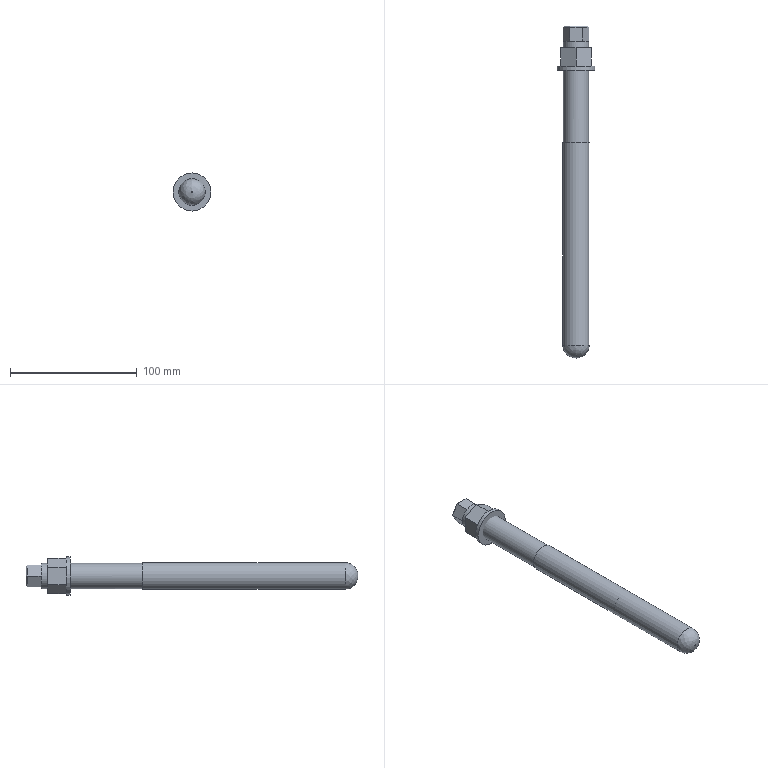Part | STEP file | Chemical anchor bolt M20X260 8.8 JBZQ4757-2006_Default<As Machined> | 4 solids | 38 faces | box 30 x 262 x 30 mm | volume 79535 mm3 | plane 33 | cylinder 4 | other 1 | commonest cylinder face diameters 19 x1 20 x1 21 x1 30 x1